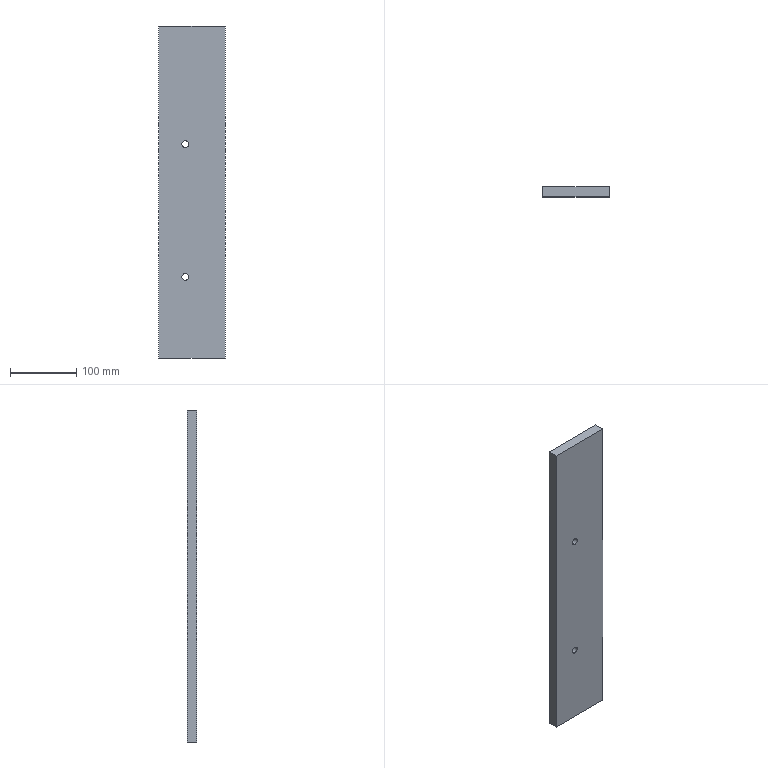Part | STEP file | Plate A | 1 solid | 10 faces | box 100 x 15 x 500 mm | volume 747549 mm3 | plane 6 | cylinder 4 | commonest cylinder face diameters 10.2 x4
STEP:
#1=CARTESIAN_POINT('',(0.,0.,0.));
#2=DIRECTION('',(0.,0.,1.));
#3=DIRECTION('',(1.,0.,0.));
#4=AXIS2_PLACEMENT_3D('',#1,#2,#3);
#5=CARTESIAN_POINT('',(-10.,7.5,-133.1));
#6=VERTEX_POINT('',#5);
#7=CARTESIAN_POINT('',(-10.,-7.5,-133.1));
#8=VERTEX_POINT('',#7);
#9=CARTESIAN_POINT('',(-10.,-7.5,-133.1));
#10=DIRECTION('',(0.,-1.,0.));
#11=VECTOR('',#10,1.);
#12=LINE('',#9,#11);
#13=CARTESIAN_POINT('',(-10.,-7.5,-128.));
#14=DIRECTION('',(0.,-1.,0.));
#15=DIRECTION('',(0.,0.,-1.));
#16=AXIS2_PLACEMENT_3D('',#13,#14,#15);
#17=CYLINDRICAL_SURFACE('',#16,5.1);
#18=CARTESIAN_POINT('',(6.283,0.));
#19=DIRECTION('',(0.,1.));
#20=VECTOR('',#19,1.);
#21=LINE('',#18,#20);
#22=(GEOMETRIC_REPRESENTATION_CONTEXT(2)PARAMETRIC_REPRESENTATION_CONTEXT()REPRESENTATION_CONTEXT('',''));
#23=DEFINITIONAL_REPRESENTATION('',(#21),#22);
#24=PCURVE('',#17,#23);
#25=CARTESIAN_POINT('',(-10.,-7.5,-128.));
#26=DIRECTION('',(0.,-1.,0.));
#27=DIRECTION('',(0.,0.,-1.));
#28=AXIS2_PLACEMENT_3D('',#25,#26,#27);
#29=CYLINDRICAL_SURFACE('',#28,5.1);
#30=CARTESIAN_POINT('',(0.,0.));
#31=DIRECTION('',(0.,1.));
#32=VECTOR('',#31,1.);
#33=LINE('',#30,#32);
#34=(GEOMETRIC_REPRESENTATION_CONTEXT(2)PARAMETRIC_REPRESENTATION_CONTEXT()REPRESENTATION_CONTEXT('',''));
#35=DEFINITIONAL_REPRESENTATION('',(#33),#34);
#36=PCURVE('',#29,#35);
#37=SURFACE_CURVE('',#12,(#24,#36),.PCURVE_S1.);
#38=EDGE_CURVE('',#6,#8,#37,.T.);
#39=ORIENTED_EDGE('',*,*,#38,.T.);
#40=CARTESIAN_POINT('',(-10.,-7.5,-122.9));
#41=VERTEX_POINT('',#40);
#42=CARTESIAN_POINT('',(-10.,-7.5,-128.));
#43=DIRECTION('',(0.,-1.,0.));
#44=DIRECTION('',(0.,0.,-1.));
#45=AXIS2_PLACEMENT_3D('',#42,#43,#44);
#46=CIRCLE('',#45,5.1);
#47=CARTESIAN_POINT('',(0.,0.));
#48=DIRECTION('',(1.,0.));
#49=VECTOR('',#48,1.);
#50=LINE('',#47,#49);
#51=(GEOMETRIC_REPRESENTATION_CONTEXT(2)PARAMETRIC_REPRESENTATION_CONTEXT()REPRESENTATION_CONTEXT('',''));
#52=DEFINITIONAL_REPRESENTATION('',(#50),#51);
#53=PCURVE('',#17,#52);
#54=CARTESIAN_POINT('',(0.,-7.5,0.));
#55=DIRECTION('',(0.,1.,0.));
#56=DIRECTION('',(0.,0.,1.));
#57=AXIS2_PLACEMENT_3D('',#54,#55,#56);
#58=PLANE('',#57);
#59=CARTESIAN_POINT('',(-133.1,-10.));
#60=CARTESIAN_POINT('',(-133.1,-1.167));
#61=CARTESIAN_POINT('',(-125.45,-5.583));
#62=CARTESIAN_POINT('',(-117.8,-10.));
#63=CARTESIAN_POINT('',(-125.45,-14.417));
#64=CARTESIAN_POINT('',(-133.1,-18.833));
#65=CARTESIAN_POINT('',(-133.1,-10.));
#66=(BOUNDED_CURVE()B_SPLINE_CURVE(2,(#59,#60,#61,#62,#63,#64,#65),.UNSPECIFIED.,.T.,.F.)B_SPLINE_CURVE_WITH_KNOTS((1,2,2,2,2,1),(-2.094,0.,2.094,4.189,6.283,8.378),.UNSPECIFIED.)CURVE()GEOMETRIC_REPRESENTATION_ITEM()RATIONAL_B_SPLINE_CURVE((1.,0.5,1.,0.5,1.,0.5,1.))REPRESENTATION_ITEM(''));
#67=(GEOMETRIC_REPRESENTATION_CONTEXT(2)PARAMETRIC_REPRESENTATION_CONTEXT()REPRESENTATION_CONTEXT('',''));
#68=DEFINITIONAL_REPRESENTATION('',(#66),#67);
#69=PCURVE('',#58,#68);
#70=SURFACE_CURVE('',#46,(#53,#69),.PCURVE_S1.);
#71=EDGE_CURVE('',#41,#8,#70,.T.);
#72=ORIENTED_EDGE('',*,*,#71,.F.);
#73=CARTESIAN_POINT('',(-10.,7.5,-122.9));
#74=VERTEX_POINT('',#73);
#75=CARTESIAN_POINT('',(-10.,-7.5,-122.9));
#76=DIRECTION('',(0.,-1.,0.));
#77=VECTOR('',#76,1.);
#78=LINE('',#75,#77);
#79=CARTESIAN_POINT('',(3.142,0.));
#80=DIRECTION('',(0.,1.));
#81=VECTOR('',#80,1.);
#82=LINE('',#79,#81);
#83=(GEOMETRIC_REPRESENTATION_CONTEXT(2)PARAMETRIC_REPRESENTATION_CONTEXT()REPRESENTATION_CONTEXT('',''));
#84=DEFINITIONAL_REPRESENTATION('',(#82),#83);
#85=PCURVE('',#17,#84);
#86=CARTESIAN_POINT('',(3.142,0.));
#87=DIRECTION('',(0.,1.));
#88=VECTOR('',#87,1.);
#89=LINE('',#86,#88);
#90=(GEOMETRIC_REPRESENTATION_CONTEXT(2)PARAMETRIC_REPRESENTATION_CONTEXT()REPRESENTATION_CONTEXT('',''));
#91=DEFINITIONAL_REPRESENTATION('',(#89),#90);
#92=PCURVE('',#29,#91);
#93=SURFACE_CURVE('',#78,(#85,#92),.PCURVE_S1.);
#94=EDGE_CURVE('',#74,#41,#93,.T.);
#95=ORIENTED_EDGE('',*,*,#94,.F.);
#96=CARTESIAN_POINT('',(-10.,7.5,-128.));
#97=DIRECTION('',(0.,-1.,0.));
#98=DIRECTION('',(0.,0.,-1.));
#99=AXIS2_PLACEMENT_3D('',#96,#97,#98);
#100=CIRCLE('',#99,5.1);
#101=CARTESIAN_POINT('',(0.,-15.));
#102=DIRECTION('',(1.,0.));
#103=VECTOR('',#102,1.);
#104=LINE('',#101,#103);
#105=(GEOMETRIC_REPRESENTATION_CONTEXT(2)PARAMETRIC_REPRESENTATION_CONTEXT()REPRESENTATION_CONTEXT('',''));
#106=DEFINITIONAL_REPRESENTATION('',(#104),#105);
#107=PCURVE('',#17,#106);
#108=CARTESIAN_POINT('',(0.,7.5,0.));
#109=DIRECTION('',(0.,1.,0.));
#110=DIRECTION('',(0.,0.,1.));
#111=AXIS2_PLACEMENT_3D('',#108,#109,#110);
#112=PLANE('',#111);
#113=CARTESIAN_POINT('',(-133.1,-10.));
#114=CARTESIAN_POINT('',(-133.1,-1.167));
#115=CARTESIAN_POINT('',(-125.45,-5.583));
#116=CARTESIAN_POINT('',(-117.8,-10.));
#117=CARTESIAN_POINT('',(-125.45,-14.417));
#118=CARTESIAN_POINT('',(-133.1,-18.833));
#119=CARTESIAN_POINT('',(-133.1,-10.));
#120=(BOUNDED_CURVE()B_SPLINE_CURVE(2,(#113,#114,#115,#116,#117,#118,#119),.UNSPECIFIED.,.T.,.F.)B_SPLINE_CURVE_WITH_KNOTS((1,2,2,2,2,1),(-2.094,0.,2.094,4.189,6.283,8.378),.UNSPECIFIED.)CURVE()GEOMETRIC_REPRESENTATION_ITEM()RATIONAL_B_SPLINE_CURVE((1.,0.5,1.,0.5,1.,0.5,1.))REPRESENTATION_ITEM(''));
#121=(GEOMETRIC_REPRESENTATION_CONTEXT(2)PARAMETRIC_REPRESENTATION_CONTEXT()REPRESENTATION_CONTEXT('',''));
#122=DEFINITIONAL_REPRESENTATION('',(#120),#121);
#123=PCURVE('',#112,#122);
#124=SURFACE_CURVE('',#100,(#107,#123),.PCURVE_S1.);
#125=EDGE_CURVE('',#74,#6,#124,.T.);
#126=ORIENTED_EDGE('',*,*,#125,.T.);
#127=EDGE_LOOP('',(#39,#72,#95,#126));
#128=FACE_BOUND('',#127,.F.);
#129=ADVANCED_FACE('',(#128),#17,.F.);
#130=CARTESIAN_POINT('',(-10.,7.5,66.9));
#131=VERTEX_POINT('',#130);
#132=CARTESIAN_POINT('',(-10.,-7.5,66.9));
#133=VERTEX_POINT('',#132);
#134=CARTESIAN_POINT('',(-10.,-7.5,66.9));
#135=DIRECTION('',(0.,-1.,0.));
#136=VECTOR('',#135,1.);
#137=LINE('',#134,#136);
#138=CARTESIAN_POINT('',(-10.,-7.5,72.));
#139=DIRECTION('',(0.,-1.,0.));
#140=DIRECTION('',(0.,0.,-1.));
#141=AXIS2_PLACEMENT_3D('',#138,#139,#140);
#142=CYLINDRICAL_SURFACE('',#141,5.1);
#143=CARTESIAN_POINT('',(6.283,0.));
#144=DIRECTION('',(0.,1.));
#145=VECTOR('',#144,1.);
#146=LINE('',#143,#145);
#147=(GEOMETRIC_REPRESENTATION_CONTEXT(2)PARAMETRIC_REPRESENTATION_CONTEXT()REPRESENTATION_CONTEXT('',''));
#148=DEFINITIONAL_REPRESENTATION('',(#146),#147);
#149=PCURVE('',#142,#148);
#150=CARTESIAN_POINT('',(-10.,-7.5,72.));
#151=DIRECTION('',(0.,-1.,0.));
#152=DIRECTION('',(0.,0.,-1.));
#153=AXIS2_PLACEMENT_3D('',#150,#151,#152);
#154=CYLINDRICAL_SURFACE('',#153,5.1);
#155=CARTESIAN_POINT('',(0.,0.));
#156=DIRECTION('',(0.,1.));
#157=VECTOR('',#156,1.);
#158=LINE('',#155,#157);
#159=(GEOMETRIC_REPRESENTATION_CONTEXT(2)PARAMETRIC_REPRESENTATION_CONTEXT()REPRESENTATION_CONTEXT('',''));
#160=DEFINITIONAL_REPRESENTATION('',(#158),#159);
#161=PCURVE('',#154,#160);
#162=SURFACE_CURVE('',#137,(#149,#161),.PCURVE_S1.);
#163=EDGE_CURVE('',#131,#133,#162,.T.);
#164=ORIENTED_EDGE('',*,*,#163,.T.);
#165=CARTESIAN_POINT('',(-10.,-7.5,77.1));
#166=VERTEX_POINT('',#165);
#167=CARTESIAN_POINT('',(-10.,-7.5,72.));
#168=DIRECTION('',(0.,-1.,0.));
#169=DIRECTION('',(0.,0.,-1.));
#170=AXIS2_PLACEMENT_3D('',#167,#168,#169);
#171=CIRCLE('',#170,5.1);
#172=CARTESIAN_POINT('',(0.,0.));
#173=DIRECTION('',(1.,0.));
#174=VECTOR('',#173,1.);
#175=LINE('',#172,#174);
#176=(GEOMETRIC_REPRESENTATION_CONTEXT(2)PARAMETRIC_REPRESENTATION_CONTEXT()REPRESENTATION_CONTEXT('',''));
#177=DEFINITIONAL_REPRESENTATION('',(#175),#176);
#178=PCURVE('',#142,#177);
#179=CARTESIAN_POINT('',(66.9,-10.));
#180=CARTESIAN_POINT('',(66.9,-1.167));
#181=CARTESIAN_POINT('',(74.55,-5.583));
#182=CARTESIAN_POINT('',(82.2,-10.));
#183=CARTESIAN_POINT('',(74.55,-14.417));
#184=CARTESIAN_POINT('',(66.9,-18.833));
#185=CARTESIAN_POINT('',(66.9,-10.));
#186=(BOUNDED_CURVE()B_SPLINE_CURVE(2,(#179,#180,#181,#182,#183,#184,#185),.UNSPECIFIED.,.T.,.F.)B_SPLINE_CURVE_WITH_KNOTS((1,2,2,2,2,1),(-2.094,0.,2.094,4.189,6.283,8.378),.UNSPECIFIED.)CURVE()GEOMETRIC_REPRESENTATION_ITEM()RATIONAL_B_SPLINE_CURVE((1.,0.5,1.,0.5,1.,0.5,1.))REPRESENTATION_ITEM(''));
#187=(GEOMETRIC_REPRESENTATION_CONTEXT(2)PARAMETRIC_REPRESENTATION_CONTEXT()REPRESENTATION_CONTEXT('',''));
#188=DEFINITIONAL_REPRESENTATION('',(#186),#187);
#189=PCURVE('',#58,#188);
#190=SURFACE_CURVE('',#171,(#178,#189),.PCURVE_S1.);
#191=EDGE_CURVE('',#166,#133,#190,.T.);
#192=ORIENTED_EDGE('',*,*,#191,.F.);
#193=CARTESIAN_POINT('',(-10.,7.5,77.1));
#194=VERTEX_POINT('',#193);
#195=CARTESIAN_POINT('',(-10.,-7.5,77.1));
#196=DIRECTION('',(0.,-1.,0.));
#197=VECTOR('',#196,1.);
#198=LINE('',#195,#197);
#199=CARTESIAN_POINT('',(3.142,0.));
#200=DIRECTION('',(0.,1.));
#201=VECTOR('',#200,1.);
#202=LINE('',#199,#201);
#203=(GEOMETRIC_REPRESENTATION_CONTEXT(2)PARAMETRIC_REPRESENTATION_CONTEXT()REPRESENTATION_CONTEXT('',''));
#204=DEFINITIONAL_REPRESENTATION('',(#202),#203);
#205=PCURVE('',#142,#204);
#206=CARTESIAN_POINT('',(3.142,0.));
#207=DIRECTION('',(0.,1.));
#208=VECTOR('',#207,1.);
#209=LINE('',#206,#208);
#210=(GEOMETRIC_REPRESENTATION_CONTEXT(2)PARAMETRIC_REPRESENTATION_CONTEXT()REPRESENTATION_CONTEXT('',''));
#211=DEFINITIONAL_REPRESENTATION('',(#209),#210);
#212=PCURVE('',#154,#211);
#213=SURFACE_CURVE('',#198,(#205,#212),.PCURVE_S1.);
#214=EDGE_CURVE('',#194,#166,#213,.T.);
#215=ORIENTED_EDGE('',*,*,#214,.F.);
#216=CARTESIAN_POINT('',(-10.,7.5,72.));
#217=DIRECTION('',(0.,-1.,0.));
#218=DIRECTION('',(0.,0.,-1.));
#219=AXIS2_PLACEMENT_3D('',#216,#217,#218);
#220=CIRCLE('',#219,5.1);
#221=CARTESIAN_POINT('',(0.,-15.));
#222=DIRECTION('',(1.,0.));
#223=VECTOR('',#222,1.);
#224=LINE('',#221,#223);
#225=(GEOMETRIC_REPRESENTATION_CONTEXT(2)PARAMETRIC_REPRESENTATION_CONTEXT()REPRESENTATION_CONTEXT('',''));
#226=DEFINITIONAL_REPRESENTATION('',(#224),#225);
#227=PCURVE('',#142,#226);
#228=CARTESIAN_POINT('',(66.9,-10.));
#229=CARTESIAN_POINT('',(66.9,-1.167));
#230=CARTESIAN_POINT('',(74.55,-5.583));
#231=CARTESIAN_POINT('',(82.2,-10.));
#232=CARTESIAN_POINT('',(74.55,-14.417));
#233=CARTESIAN_POINT('',(66.9,-18.833));
#234=CARTESIAN_POINT('',(66.9,-10.));
#235=(BOUNDED_CURVE()B_SPLINE_CURVE(2,(#228,#229,#230,#231,#232,#233,#234),.UNSPECIFIED.,.T.,.F.)B_SPLINE_CURVE_WITH_KNOTS((1,2,2,2,2,1),(-2.094,0.,2.094,4.189,6.283,8.378),.UNSPECIFIED.)CURVE()GEOMETRIC_REPRESENTATION_ITEM()RATIONAL_B_SPLINE_CURVE((1.,0.5,1.,0.5,1.,0.5,1.))REPRESENTATION_ITEM(''));
#236=(GEOMETRIC_REPRESENTATION_CONTEXT(2)PARAMETRIC_REPRESENTATION_CONTEXT()REPRESENTATION_CONTEXT('',''));
#237=DEFINITIONAL_REPRESENTATION('',(#235),#236);
#238=PCURVE('',#112,#237);
#239=SURFACE_CURVE('',#220,(#227,#238),.PCURVE_S1.);
#240=EDGE_CURVE('',#194,#131,#239,.T.);
#241=ORIENTED_EDGE('',*,*,#240,.T.);
#242=EDGE_LOOP('',(#164,#192,#215,#241));
#243=FACE_BOUND('',#242,.F.);
#244=ADVANCED_FACE('',(#243),#142,.F.);
#245=CARTESIAN_POINT('',(50.,7.5,250.));
#246=VERTEX_POINT('',#245);
#247=CARTESIAN_POINT('',(50.,7.5,-250.));
#248=VERTEX_POINT('',#247);
#249=CARTESIAN_POINT('',(50.,7.5,-250.));
#250=DIRECTION('',(0.,0.,-1.));
#251=VECTOR('',#250,1.);
#252=LINE('',#249,#251);
#253=CARTESIAN_POINT('',(-250.,50.));
#254=DIRECTION('',(-1.,0.));
#255=VECTOR('',#254,1.);
#256=LINE('',#253,#255);
#257=(GEOMETRIC_REPRESENTATION_CONTEXT(2)PARAMETRIC_REPRESENTATION_CONTEXT()REPRESENTATION_CONTEXT('',''));
#258=DEFINITIONAL_REPRESENTATION('',(#256),#257);
#259=PCURVE('',#112,#258);
#260=CARTESIAN_POINT('',(50.,7.5,-250.));
#261=DIRECTION('',(-1.,0.,0.));
#262=DIRECTION('',(0.,0.,1.));
#263=AXIS2_PLACEMENT_3D('',#260,#261,#262);
#264=PLANE('',#263);
#265=CARTESIAN_POINT('',(0.,0.));
#266=DIRECTION('',(-1.,0.));
#267=VECTOR('',#266,1.);
#268=LINE('',#265,#267);
#269=(GEOMETRIC_REPRESENTATION_CONTEXT(2)PARAMETRIC_REPRESENTATION_CONTEXT()REPRESENTATION_CONTEXT('',''));
#270=DEFINITIONAL_REPRESENTATION('',(#268),#269);
#271=PCURVE('',#264,#270);
#272=SURFACE_CURVE('',#252,(#259,#271),.PCURVE_S1.);
#273=EDGE_CURVE('',#246,#248,#272,.T.);
#274=ORIENTED_EDGE('',*,*,#273,.T.);
#275=CARTESIAN_POINT('',(-50.,7.5,-250.));
#276=VERTEX_POINT('',#275);
#277=CARTESIAN_POINT('',(-50.,7.5,-250.));
#278=DIRECTION('',(-1.,0.,0.));
#279=VECTOR('',#278,1.);
#280=LINE('',#277,#279);
#281=CARTESIAN_POINT('',(-250.,-50.));
#282=DIRECTION('',(0.,-1.));
#283=VECTOR('',#282,1.);
#284=LINE('',#281,#283);
#285=(GEOMETRIC_REPRESENTATION_CONTEXT(2)PARAMETRIC_REPRESENTATION_CONTEXT()REPRESENTATION_CONTEXT('',''));
#286=DEFINITIONAL_REPRESENTATION('',(#284),#285);
#287=PCURVE('',#112,#286);
#288=CARTESIAN_POINT('',(-50.,7.5,-250.));
#289=DIRECTION('',(0.,0.,1.));
#290=DIRECTION('',(1.,0.,0.));
#291=AXIS2_PLACEMENT_3D('',#288,#289,#290);
#292=PLANE('',#291);
#293=CARTESIAN_POINT('',(0.,0.));
#294=DIRECTION('',(-1.,0.));
#295=VECTOR('',#294,1.);
#296=LINE('',#293,#295);
#297=(GEOMETRIC_REPRESENTATION_CONTEXT(2)PARAMETRIC_REPRESENTATION_CONTEXT()REPRESENTATION_CONTEXT('',''));
#298=DEFINITIONAL_REPRESENTATION('',(#296),#297);
#299=PCURVE('',#292,#298);
#300=SURFACE_CURVE('',#280,(#287,#299),.PCURVE_S1.);
#301=EDGE_CURVE('',#248,#276,#300,.T.);
#302=ORIENTED_EDGE('',*,*,#301,.T.);
#303=CARTESIAN_POINT('',(-50.,7.5,250.));
#304=VERTEX_POINT('',#303);
#305=CARTESIAN_POINT('',(-50.,7.5,-250.));
#306=DIRECTION('',(0.,0.,1.));
#307=VECTOR('',#306,1.);
#308=LINE('',#305,#307);
#309=CARTESIAN_POINT('',(-250.,-50.));
#310=DIRECTION('',(1.,0.));
#311=VECTOR('',#310,1.);
#312=LINE('',#309,#311);
#313=(GEOMETRIC_REPRESENTATION_CONTEXT(2)PARAMETRIC_REPRESENTATION_CONTEXT()REPRESENTATION_CONTEXT('',''));
#314=DEFINITIONAL_REPRESENTATION('',(#312),#313);
#315=PCURVE('',#112,#314);
#316=CARTESIAN_POINT('',(-50.,7.5,-250.));
#317=DIRECTION('',(1.,0.,0.));
#318=DIRECTION('',(0.,0.,-1.));
#319=AXIS2_PLACEMENT_3D('',#316,#317,#318);
#320=PLANE('',#319);
#321=CARTESIAN_POINT('',(0.,0.));
#322=DIRECTION('',(-1.,0.));
#323=VECTOR('',#322,1.);
#324=LINE('',#321,#323);
#325=(GEOMETRIC_REPRESENTATION_CONTEXT(2)PARAMETRIC_REPRESENTATION_CONTEXT()REPRESENTATION_CONTEXT('',''));
#326=DEFINITIONAL_REPRESENTATION('',(#324),#325);
#327=PCURVE('',#320,#326);
#328=SURFACE_CURVE('',#308,(#315,#327),.PCURVE_S1.);
#329=EDGE_CURVE('',#276,#304,#328,.T.);
#330=ORIENTED_EDGE('',*,*,#329,.T.);
#331=CARTESIAN_POINT('',(-50.,7.5,250.));
#332=DIRECTION('',(1.,0.,0.));
#333=VECTOR('',#332,1.);
#334=LINE('',#331,#333);
#335=CARTESIAN_POINT('',(250.,-50.));
#336=DIRECTION('',(0.,1.));
#337=VECTOR('',#336,1.);
#338=LINE('',#335,#337);
#339=(GEOMETRIC_REPRESENTATION_CONTEXT(2)PARAMETRIC_REPRESENTATION_CONTEXT()REPRESENTATION_CONTEXT('',''));
#340=DEFINITIONAL_REPRESENTATION('',(#338),#339);
#341=PCURVE('',#112,#340);
#342=CARTESIAN_POINT('',(-50.,7.5,250.));
#343=DIRECTION('',(0.,0.,-1.));
#344=DIRECTION('',(-1.,0.,0.));
#345=AXIS2_PLACEMENT_3D('',#342,#343,#344);
#346=PLANE('',#345);
#347=CARTESIAN_POINT('',(0.,0.));
#348=DIRECTION('',(-1.,0.));
#349=VECTOR('',#348,1.);
#350=LINE('',#347,#349);
#351=(GEOMETRIC_REPRESENTATION_CONTEXT(2)PARAMETRIC_REPRESENTATION_CONTEXT()REPRESENTATION_CONTEXT('',''));
#352=DEFINITIONAL_REPRESENTATION('',(#350),#351);
#353=PCURVE('',#346,#352);
#354=SURFACE_CURVE('',#334,(#341,#353),.PCURVE_S1.);
#355=EDGE_CURVE('',#304,#246,#354,.T.);
#356=ORIENTED_EDGE('',*,*,#355,.T.);
#357=EDGE_LOOP('',(#274,#302,#330,#356));
#358=FACE_BOUND('',#357,.T.);
#359=CARTESIAN_POINT('',(-10.,7.5,72.));
#360=DIRECTION('',(0.,-1.,0.));
#361=DIRECTION('',(0.,0.,-1.));
#362=AXIS2_PLACEMENT_3D('',#359,#360,#361);
#363=CIRCLE('',#362,5.1);
#364=CARTESIAN_POINT('',(66.9,-10.));
#365=CARTESIAN_POINT('',(66.9,-1.167));
#366=CARTESIAN_POINT('',(74.55,-5.583));
#367=CARTESIAN_POINT('',(82.2,-10.));
#368=CARTESIAN_POINT('',(74.55,-14.417));
#369=CARTESIAN_POINT('',(66.9,-18.833));
#370=CARTESIAN_POINT('',(66.9,-10.));
#371=(BOUNDED_CURVE()B_SPLINE_CURVE(2,(#364,#365,#366,#367,#368,#369,#370),.UNSPECIFIED.,.T.,.F.)B_SPLINE_CURVE_WITH_KNOTS((1,2,2,2,2,1),(-2.094,0.,2.094,4.189,6.283,8.378),.UNSPECIFIED.)CURVE()GEOMETRIC_REPRESENTATION_ITEM()RATIONAL_B_SPLINE_CURVE((1.,0.5,1.,0.5,1.,0.5,1.))REPRESENTATION_ITEM(''));
#372=(GEOMETRIC_REPRESENTATION_CONTEXT(2)PARAMETRIC_REPRESENTATION_CONTEXT()REPRESENTATION_CONTEXT('',''));
#373=DEFINITIONAL_REPRESENTATION('',(#371),#372);
#374=PCURVE('',#112,#373);
#375=CARTESIAN_POINT('',(0.,-15.));
#376=DIRECTION('',(1.,0.));
#377=VECTOR('',#376,1.);
#378=LINE('',#375,#377);
#379=(GEOMETRIC_REPRESENTATION_CONTEXT(2)PARAMETRIC_REPRESENTATION_CONTEXT()REPRESENTATION_CONTEXT('',''));
#380=DEFINITIONAL_REPRESENTATION('',(#378),#379);
#381=PCURVE('',#154,#380);
#382=SURFACE_CURVE('',#363,(#374,#381),.PCURVE_S1.);
#383=EDGE_CURVE('',#131,#194,#382,.T.);
#384=ORIENTED_EDGE('',*,*,#383,.T.);
#385=ORIENTED_EDGE('',*,*,#240,.T.);
#386=EDGE_LOOP('',(#384,#385));
#387=FACE_BOUND('',#386,.T.);
#388=CARTESIAN_POINT('',(-10.,7.5,-128.));
#389=DIRECTION('',(0.,-1.,0.));
#390=DIRECTION('',(0.,0.,-1.));
#391=AXIS2_PLACEMENT_3D('',#388,#389,#390);
#392=CIRCLE('',#391,5.1);
#393=CARTESIAN_POINT('',(-133.1,-10.));
#394=CARTESIAN_POINT('',(-133.1,-1.167));
#395=CARTESIAN_POINT('',(-125.45,-5.583));
#396=CARTESIAN_POINT('',(-117.8,-10.));
#397=CARTESIAN_POINT('',(-125.45,-14.417));
#398=CARTESIAN_POINT('',(-133.1,-18.833));
#399=CARTESIAN_POINT('',(-133.1,-10.));
#400=(BOUNDED_CURVE()B_SPLINE_CURVE(2,(#393,#394,#395,#396,#397,#398,#399),.UNSPECIFIED.,.T.,.F.)B_SPLINE_CURVE_WITH_KNOTS((1,2,2,2,2,1),(-2.094,0.,2.094,4.189,6.283,8.378),.UNSPECIFIED.)CURVE()GEOMETRIC_REPRESENTATION_ITEM()RATIONAL_B_SPLINE_CURVE((1.,0.5,1.,0.5,1.,0.5,1.))REPRESENTATION_ITEM(''));
#401=(GEOMETRIC_REPRESENTATION_CONTEXT(2)PARAMETRIC_REPRESENTATION_CONTEXT()REPRESENTATION_CONTEXT('',''));
#402=DEFINITIONAL_REPRESENTATION('',(#400),#401);
#403=PCURVE('',#112,#402);
#404=CARTESIAN_POINT('',(0.,-15.));
#405=DIRECTION('',(1.,0.));
#406=VECTOR('',#405,1.);
#407=LINE('',#404,#406);
#408=(GEOMETRIC_REPRESENTATION_CONTEXT(2)PARAMETRIC_REPRESENTATION_CONTEXT()REPRESENTATION_CONTEXT('',''));
#409=DEFINITIONAL_REPRESENTATION('',(#407),#408);
#410=PCURVE('',#29,#409);
#411=SURFACE_CURVE('',#392,(#403,#410),.PCURVE_S1.);
#412=EDGE_CURVE('',#6,#74,#411,.T.);
#413=ORIENTED_EDGE('',*,*,#412,.T.);
#414=ORIENTED_EDGE('',*,*,#125,.T.);
#415=EDGE_LOOP('',(#413,#414));
#416=FACE_BOUND('',#415,.T.);
#417=ADVANCED_FACE('',(#358,#387,#416),#112,.T.);
#418=CARTESIAN_POINT('',(-10.,-7.5,-128.));
#419=DIRECTION('',(0.,-1.,0.));
#420=DIRECTION('',(0.,0.,-1.));
#421=AXIS2_PLACEMENT_3D('',#418,#419,#420);
#422=CIRCLE('',#421,5.1);
#423=CARTESIAN_POINT('',(-133.1,-10.));
#424=CARTESIAN_POINT('',(-133.1,-1.167));
#425=CARTESIAN_POINT('',(-125.45,-5.583));
#426=CARTESIAN_POINT('',(-117.8,-10.));
#427=CARTESIAN_POINT('',(-125.45,-14.417));
#428=CARTESIAN_POINT('',(-133.1,-18.833));
#429=CARTESIAN_POINT('',(-133.1,-10.));
#430=(BOUNDED_CURVE()B_SPLINE_CURVE(2,(#423,#424,#425,#426,#427,#428,#429),.UNSPECIFIED.,.T.,.F.)B_SPLINE_CURVE_WITH_KNOTS((1,2,2,2,2,1),(-2.094,0.,2.094,4.189,6.283,8.378),.UNSPECIFIED.)CURVE()GEOMETRIC_REPRESENTATION_ITEM()RATIONAL_B_SPLINE_CURVE((1.,0.5,1.,0.5,1.,0.5,1.))REPRESENTATION_ITEM(''));
#431=(GEOMETRIC_REPRESENTATION_CONTEXT(2)PARAMETRIC_REPRESENTATION_CONTEXT()REPRESENTATION_CONTEXT('',''));
#432=DEFINITIONAL_REPRESENTATION('',(#430),#431);
#433=PCURVE('',#58,#432);
#434=CARTESIAN_POINT('',(0.,0.));
#435=DIRECTION('',(1.,0.));
#436=VECTOR('',#435,1.);
#437=LINE('',#434,#436);
#438=(GEOMETRIC_REPRESENTATION_CONTEXT(2)PARAMETRIC_REPRESENTATION_CONTEXT()REPRESENTATION_CONTEXT('',''));
#439=DEFINITIONAL_REPRESENTATION('',(#437),#438);
#440=PCURVE('',#29,#439);
#441=SURFACE_CURVE('',#422,(#433,#440),.PCURVE_S1.);
#442=EDGE_CURVE('',#8,#41,#441,.T.);
#443=ORIENTED_EDGE('',*,*,#442,.F.);
#444=ORIENTED_EDGE('',*,*,#71,.F.);
#445=EDGE_LOOP('',(#443,#444));
#446=FACE_BOUND('',#445,.T.);
#447=CARTESIAN_POINT('',(50.,-7.5,250.));
#448=VERTEX_POINT('',#447);
#449=CARTESIAN_POINT('',(50.,-7.5,-250.));
#450=VERTEX_POINT('',#449);
#451=CARTESIAN_POINT('',(50.,-7.5,-250.));
#452=DIRECTION('',(0.,0.,-1.));
#453=VECTOR('',#452,1.);
#454=LINE('',#451,#453);
#455=CARTESIAN_POINT('',(-250.,50.));
#456=DIRECTION('',(-1.,0.));
#457=VECTOR('',#456,1.);
#458=LINE('',#455,#457);
#459=(GEOMETRIC_REPRESENTATION_CONTEXT(2)PARAMETRIC_REPRESENTATION_CONTEXT()REPRESENTATION_CONTEXT('',''));
#460=DEFINITIONAL_REPRESENTATION('',(#458),#459);
#461=PCURVE('',#58,#460);
#462=CARTESIAN_POINT('',(0.,-15.));
#463=DIRECTION('',(-1.,0.));
#464=VECTOR('',#463,1.);
#465=LINE('',#462,#464);
#466=(GEOMETRIC_REPRESENTATION_CONTEXT(2)PARAMETRIC_REPRESENTATION_CONTEXT()REPRESENTATION_CONTEXT('',''));
#467=DEFINITIONAL_REPRESENTATION('',(#465),#466);
#468=PCURVE('',#264,#467);
#469=SURFACE_CURVE('',#454,(#461,#468),.PCURVE_S1.);
#470=EDGE_CURVE('',#448,#450,#469,.T.);
#471=ORIENTED_EDGE('',*,*,#470,.F.);
#472=CARTESIAN_POINT('',(-50.,-7.5,250.));
#473=VERTEX_POINT('',#472);
#474=CARTESIAN_POINT('',(-50.,-7.5,250.));
#475=DIRECTION('',(1.,0.,0.));
#476=VECTOR('',#475,1.);
#477=LINE('',#474,#476);
#478=CARTESIAN_POINT('',(250.,-50.));
#479=DIRECTION('',(0.,1.));
#480=VECTOR('',#479,1.);
#481=LINE('',#478,#480);
#482=(GEOMETRIC_REPRESENTATION_CONTEXT(2)PARAMETRIC_REPRESENTATION_CONTEXT()REPRESENTATION_CONTEXT('',''));
#483=DEFINITIONAL_REPRESENTATION('',(#481),#482);
#484=PCURVE('',#58,#483);
#485=CARTESIAN_POINT('',(0.,-15.));
#486=DIRECTION('',(-1.,0.));
#487=VECTOR('',#486,1.);
#488=LINE('',#485,#487);
#489=(GEOMETRIC_REPRESENTATION_CONTEXT(2)PARAMETRIC_REPRESENTATION_CONTEXT()REPRESENTATION_CONTEXT('',''));
#490=DEFINITIONAL_REPRESENTATION('',(#488),#489);
#491=PCURVE('',#346,#490);
#492=SURFACE_CURVE('',#477,(#484,#491),.PCURVE_S1.);
#493=EDGE_CURVE('',#473,#448,#492,.T.);
#494=ORIENTED_EDGE('',*,*,#493,.F.);
#495=CARTESIAN_POINT('',(-50.,-7.5,-250.));
#496=VERTEX_POINT('',#495);
#497=CARTESIAN_POINT('',(-50.,-7.5,-250.));
#498=DIRECTION('',(0.,0.,1.));
#499=VECTOR('',#498,1.);
#500=LINE('',#497,#499);
#501=CARTESIAN_POINT('',(-250.,-50.));
#502=DIRECTION('',(1.,0.));
#503=VECTOR('',#502,1.);
#504=LINE('',#501,#503);
#505=(GEOMETRIC_REPRESENTATION_CONTEXT(2)PARAMETRIC_REPRESENTATION_CONTEXT()REPRESENTATION_CONTEXT('',''));
#506=DEFINITIONAL_REPRESENTATION('',(#504),#505);
#507=PCURVE('',#58,#506);
#508=CARTESIAN_POINT('',(0.,-15.));
#509=DIRECTION('',(-1.,0.));
#510=VECTOR('',#509,1.);
#511=LINE('',#508,#510);
#512=(GEOMETRIC_REPRESENTATION_CONTEXT(2)PARAMETRIC_REPRESENTATION_CONTEXT()REPRESENTATION_CONTEXT('',''));
#513=DEFINITIONAL_REPRESENTATION('',(#511),#512);
#514=PCURVE('',#320,#513);
#515=SURFACE_CURVE('',#500,(#507,#514),.PCURVE_S1.);
#516=EDGE_CURVE('',#496,#473,#515,.T.);
#517=ORIENTED_EDGE('',*,*,#516,.F.);
#518=CARTESIAN_POINT('',(-50.,-7.5,-250.));
#519=DIRECTION('',(-1.,0.,0.));
#520=VECTOR('',#519,1.);
#521=LINE('',#518,#520);
#522=CARTESIAN_POINT('',(-250.,-50.));
#523=DIRECTION('',(0.,-1.));
#524=VECTOR('',#523,1.);
#525=LINE('',#522,#524);
#526=(GEOMETRIC_REPRESENTATION_CONTEXT(2)PARAMETRIC_REPRESENTATION_CONTEXT()REPRESENTATION_CONTEXT('',''));
#527=DEFINITIONAL_REPRESENTATION('',(#525),#526);
#528=PCURVE('',#58,#527);
#529=CARTESIAN_POINT('',(0.,-15.));
#530=DIRECTION('',(-1.,0.));
#531=VECTOR('',#530,1.);
#532=LINE('',#529,#531);
#533=(GEOMETRIC_REPRESENTATION_CONTEXT(2)PARAMETRIC_REPRESENTATION_CONTEXT()REPRESENTATION_CONTEXT('',''));
#534=DEFINITIONAL_REPRESENTATION('',(#532),#533);
#535=PCURVE('',#292,#534);
#536=SURFACE_CURVE('',#521,(#528,#535),.PCURVE_S1.);
#537=EDGE_CURVE('',#450,#496,#536,.T.);
#538=ORIENTED_EDGE('',*,*,#537,.F.);
#539=EDGE_LOOP('',(#471,#494,#517,#538));
#540=FACE_BOUND('',#539,.T.);
#541=CARTESIAN_POINT('',(-10.,-7.5,72.));
#542=DIRECTION('',(0.,-1.,0.));
#543=DIRECTION('',(0.,0.,-1.));
#544=AXIS2_PLACEMENT_3D('',#541,#542,#543);
#545=CIRCLE('',#544,5.1);
#546=CARTESIAN_POINT('',(66.9,-10.));
#547=CARTESIAN_POINT('',(66.9,-1.167));
#548=CARTESIAN_POINT('',(74.55,-5.583));
#549=CARTESIAN_POINT('',(82.2,-10.));
#550=CARTESIAN_POINT('',(74.55,-14.417));
#551=CARTESIAN_POINT('',(66.9,-18.833));
#552=CARTESIAN_POINT('',(66.9,-10.));
#553=(BOUNDED_CURVE()B_SPLINE_CURVE(2,(#546,#547,#548,#549,#550,#551,#552),.UNSPECIFIED.,.T.,.F.)B_SPLINE_CURVE_WITH_KNOTS((1,2,2,2,2,1),(-2.094,0.,2.094,4.189,6.283,8.378),.UNSPECIFIED.)CURVE()GEOMETRIC_REPRESENTATION_ITEM()RATIONAL_B_SPLINE_CURVE((1.,0.5,1.,0.5,1.,0.5,1.))REPRESENTATION_ITEM(''));
#554=(GEOMETRIC_REPRESENTATION_CONTEXT(2)PARAMETRIC_REPRESENTATION_CONTEXT()REPRESENTATION_CONTEXT('',''));
#555=DEFINITIONAL_REPRESENTATION('',(#553),#554);
#556=PCURVE('',#58,#555);
#557=CARTESIAN_POINT('',(0.,0.));
#558=DIRECTION('',(1.,0.));
#559=VECTOR('',#558,1.);
#560=LINE('',#557,#559);
#561=(GEOMETRIC_REPRESENTATION_CONTEXT(2)PARAMETRIC_REPRESENTATION_CONTEXT()REPRESENTATION_CONTEXT('',''));
#562=DEFINITIONAL_REPRESENTATION('',(#560),#561);
#563=PCURVE('',#154,#562);
#564=SURFACE_CURVE('',#545,(#556,#563),.PCURVE_S1.);
#565=EDGE_CURVE('',#133,#166,#564,.T.);
#566=ORIENTED_EDGE('',*,*,#565,.F.);
#567=ORIENTED_EDGE('',*,*,#191,.F.);
#568=EDGE_LOOP('',(#566,#567));
#569=FACE_BOUND('',#568,.T.);
#570=ADVANCED_FACE('',(#446,#540,#569),#58,.F.);
#571=ORIENTED_EDGE('',*,*,#470,.T.);
#572=CARTESIAN_POINT('',(50.,7.5,-250.));
#573=DIRECTION('',(0.,-1.,0.));
#574=VECTOR('',#573,1.);
#575=LINE('',#572,#574);
#576=CARTESIAN_POINT('',(0.,0.));
#577=DIRECTION('',(0.,-1.));
#578=VECTOR('',#577,1.);
#579=LINE('',#576,#578);
#580=(GEOMETRIC_REPRESENTATION_CONTEXT(2)PARAMETRIC_REPRESENTATION_CONTEXT()REPRESENTATION_CONTEXT('',''));
#581=DEFINITIONAL_REPRESENTATION('',(#579),#580);
#582=PCURVE('',#264,#581);
#583=CARTESIAN_POINT('',(100.,0.));
#584=DIRECTION('',(0.,-1.));
#585=VECTOR('',#584,1.);
#586=LINE('',#583,#585);
#587=(GEOMETRIC_REPRESENTATION_CONTEXT(2)PARAMETRIC_REPRESENTATION_CONTEXT()REPRESENTATION_CONTEXT('',''));
#588=DEFINITIONAL_REPRESENTATION('',(#586),#587);
#589=PCURVE('',#292,#588);
#590=SURFACE_CURVE('',#575,(#582,#589),.PCURVE_S1.);
#591=EDGE_CURVE('',#248,#450,#590,.T.);
#592=ORIENTED_EDGE('',*,*,#591,.F.);
#593=ORIENTED_EDGE('',*,*,#273,.F.);
#594=CARTESIAN_POINT('',(50.,7.5,250.));
#595=DIRECTION('',(0.,-1.,0.));
#596=VECTOR('',#595,1.);
#597=LINE('',#594,#596);
#598=CARTESIAN_POINT('',(500.,0.));
#599=DIRECTION('',(0.,-1.));
#600=VECTOR('',#599,1.);
#601=LINE('',#598,#600);
#602=(GEOMETRIC_REPRESENTATION_CONTEXT(2)PARAMETRIC_REPRESENTATION_CONTEXT()REPRESENTATION_CONTEXT('',''));
#603=DEFINITIONAL_REPRESENTATION('',(#601),#602);
#604=PCURVE('',#264,#603);
#605=CARTESIAN_POINT('',(-100.,0.));
#606=DIRECTION('',(0.,-1.));
#607=VECTOR('',#606,1.);
#608=LINE('',#605,#607);
#609=(GEOMETRIC_REPRESENTATION_CONTEXT(2)PARAMETRIC_REPRESENTATION_CONTEXT()REPRESENTATION_CONTEXT('',''));
#610=DEFINITIONAL_REPRESENTATION('',(#608),#609);
#611=PCURVE('',#346,#610);
#612=SURFACE_CURVE('',#597,(#604,#611),.PCURVE_S1.);
#613=EDGE_CURVE('',#246,#448,#612,.T.);
#614=ORIENTED_EDGE('',*,*,#613,.T.);
#615=EDGE_LOOP('',(#571,#592,#593,#614));
#616=FACE_BOUND('',#615,.T.);
#617=ADVANCED_FACE('',(#616),#264,.F.);
#618=ORIENTED_EDGE('',*,*,#537,.T.);
#619=CARTESIAN_POINT('',(-50.,7.5,-250.));
#620=DIRECTION('',(0.,-1.,0.));
#621=VECTOR('',#620,1.);
#622=LINE('',#619,#621);
#623=CARTESIAN_POINT('',(0.,0.));
#624=DIRECTION('',(0.,-1.));
#625=VECTOR('',#624,1.);
#626=LINE('',#623,#625);
#627=(GEOMETRIC_REPRESENTATION_CONTEXT(2)PARAMETRIC_REPRESENTATION_CONTEXT()REPRESENTATION_CONTEXT('',''));
#628=DEFINITIONAL_REPRESENTATION('',(#626),#627);
#629=PCURVE('',#292,#628);
#630=CARTESIAN_POINT('',(0.,0.));
#631=DIRECTION('',(0.,-1.));
#632=VECTOR('',#631,1.);
#633=LINE('',#630,#632);
#634=(GEOMETRIC_REPRESENTATION_CONTEXT(2)PARAMETRIC_REPRESENTATION_CONTEXT()REPRESENTATION_CONTEXT('',''));
#635=DEFINITIONAL_REPRESENTATION('',(#633),#634);
#636=PCURVE('',#320,#635);
#637=SURFACE_CURVE('',#622,(#629,#636),.PCURVE_S1.);
#638=EDGE_CURVE('',#276,#496,#637,.T.);
#639=ORIENTED_EDGE('',*,*,#638,.F.);
#640=ORIENTED_EDGE('',*,*,#301,.F.);
#641=ORIENTED_EDGE('',*,*,#591,.T.);
#642=EDGE_LOOP('',(#618,#639,#640,#641));
#643=FACE_BOUND('',#642,.T.);
#644=ADVANCED_FACE('',(#643),#292,.F.);
#645=ORIENTED_EDGE('',*,*,#516,.T.);
#646=CARTESIAN_POINT('',(-50.,7.5,250.));
#647=DIRECTION('',(0.,-1.,0.));
#648=VECTOR('',#647,1.);
#649=LINE('',#646,#648);
#650=CARTESIAN_POINT('',(-500.,0.));
#651=DIRECTION('',(0.,-1.));
#652=VECTOR('',#651,1.);
#653=LINE('',#650,#652);
#654=(GEOMETRIC_REPRESENTATION_CONTEXT(2)PARAMETRIC_REPRESENTATION_CONTEXT()REPRESENTATION_CONTEXT('',''));
#655=DEFINITIONAL_REPRESENTATION('',(#653),#654);
#656=PCURVE('',#320,#655);
#657=CARTESIAN_POINT('',(0.,0.));
#658=DIRECTION('',(0.,-1.));
#659=VECTOR('',#658,1.);
#660=LINE('',#657,#659);
#661=(GEOMETRIC_REPRESENTATION_CONTEXT(2)PARAMETRIC_REPRESENTATION_CONTEXT()REPRESENTATION_CONTEXT('',''));
#662=DEFINITIONAL_REPRESENTATION('',(#660),#661);
#663=PCURVE('',#346,#662);
#664=SURFACE_CURVE('',#649,(#656,#663),.PCURVE_S1.);
#665=EDGE_CURVE('',#304,#473,#664,.T.);
#666=ORIENTED_EDGE('',*,*,#665,.F.);
#667=ORIENTED_EDGE('',*,*,#329,.F.);
#668=ORIENTED_EDGE('',*,*,#638,.T.);
#669=EDGE_LOOP('',(#645,#666,#667,#668));
#670=FACE_BOUND('',#669,.T.);
#671=ADVANCED_FACE('',(#670),#320,.F.);
#672=ORIENTED_EDGE('',*,*,#493,.T.);
#673=ORIENTED_EDGE('',*,*,#613,.F.);
#674=ORIENTED_EDGE('',*,*,#355,.F.);
#675=ORIENTED_EDGE('',*,*,#665,.T.);
#676=EDGE_LOOP('',(#672,#673,#674,#675));
#677=FACE_BOUND('',#676,.T.);
#678=ADVANCED_FACE('',(#677),#346,.F.);
#679=ORIENTED_EDGE('',*,*,#565,.F.);
#680=ORIENTED_EDGE('',*,*,#163,.F.);
#681=ORIENTED_EDGE('',*,*,#383,.T.);
#682=ORIENTED_EDGE('',*,*,#214,.T.);
#683=EDGE_LOOP('',(#679,#680,#681,#682));
#684=FACE_BOUND('',#683,.F.);
#685=ADVANCED_FACE('',(#684),#154,.F.);
#686=ORIENTED_EDGE('',*,*,#442,.F.);
#687=ORIENTED_EDGE('',*,*,#38,.F.);
#688=ORIENTED_EDGE('',*,*,#412,.T.);
#689=ORIENTED_EDGE('',*,*,#94,.T.);
#690=EDGE_LOOP('',(#686,#687,#688,#689));
#691=FACE_BOUND('',#690,.F.);
#692=ADVANCED_FACE('',(#691),#29,.F.);
#693=CLOSED_SHELL('',(#129,#244,#417,#570,#617,#644,#671,#678,#685,#692));
#694=MANIFOLD_SOLID_BREP('',#693);
#695=(LENGTH_UNIT()NAMED_UNIT(*)SI_UNIT(.MILLI.,.METRE.));
#696=UNCERTAINTY_MEASURE_WITH_UNIT(LENGTH_MEASURE(0.0000001),#695,'','');
#697=(NAMED_UNIT(*)PLANE_ANGLE_UNIT()SI_UNIT($,.RADIAN.));
#698=(NAMED_UNIT(*)SI_UNIT($,.STERADIAN.)SOLID_ANGLE_UNIT());
#699=(GEOMETRIC_REPRESENTATION_CONTEXT(3)GLOBAL_UNCERTAINTY_ASSIGNED_CONTEXT((#696))GLOBAL_UNIT_ASSIGNED_CONTEXT((#695,#697,#698))REPRESENTATION_CONTEXT('',''));
#700=ADVANCED_BREP_SHAPE_REPRESENTATION('',(#4,#694),#699);